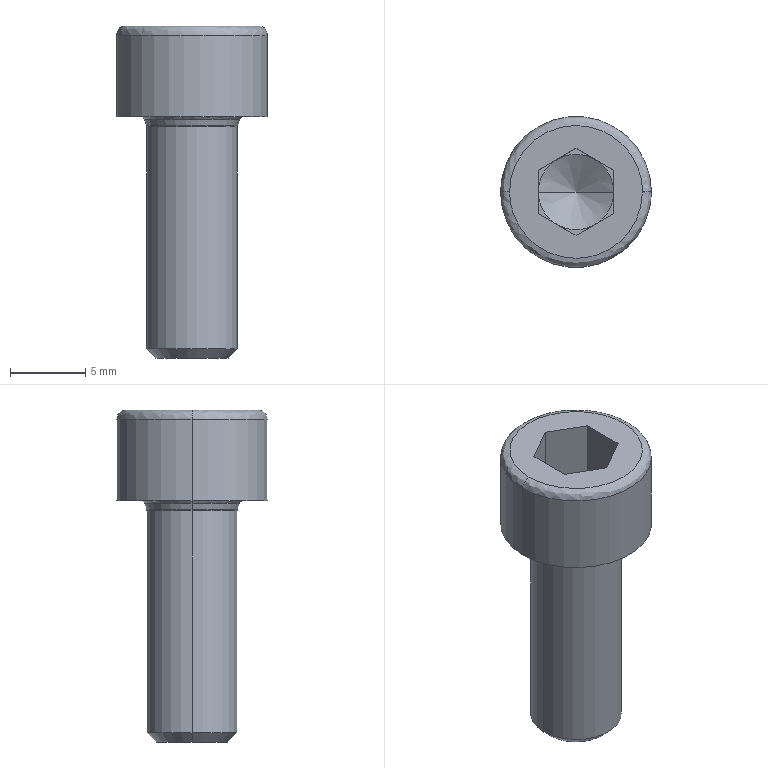Part | STEP file | 0232_Z_SSCSPD15_2 | 1 solid | 31 faces | box 10 x 10 x 22 mm | volume 829.902 mm3 | plane 15 | spline 6 | cone 6 | cylinder 4 | commonest cylinder face diameters 6 x2 10 x2